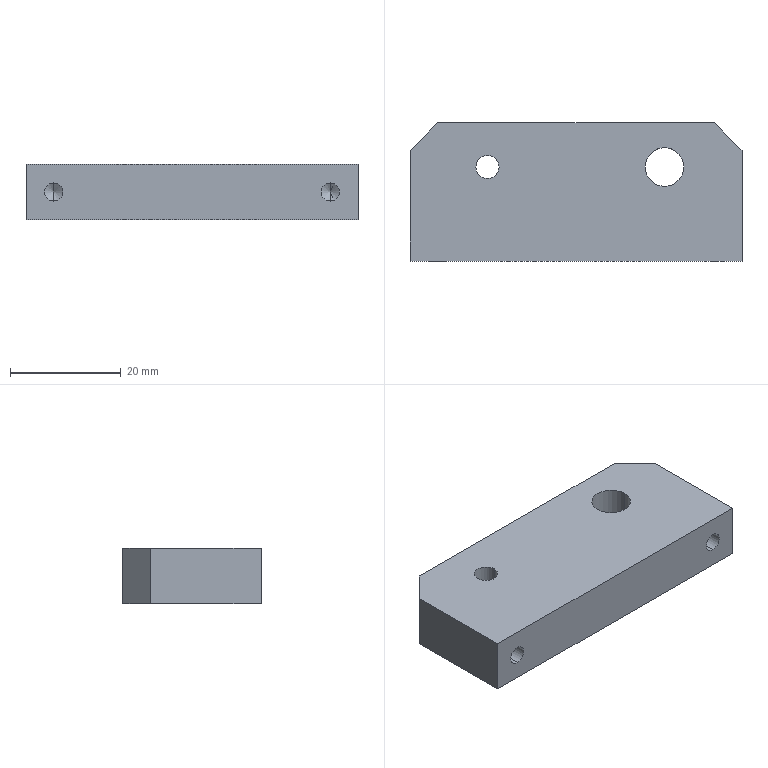Part | STEP file | PN_0049 Mount electronic clip cylinder mounting plate 2 | 1 solid | 20 faces | box 60 x 25 x 10 mm | volume 13990 mm3 | cylinder 8 | plane 8 | cone 4 | commonest cylinder face diameters 3.3 x4 4.2 x2 7 x2
STEP:
#1=CARTESIAN_POINT('',(0.,0.,0.));
#2=DIRECTION('',(0.,0.,1.));
#3=DIRECTION('',(1.,0.,0.));
#4=AXIS2_PLACEMENT_3D('',#1,#2,#3);
#5=CARTESIAN_POINT('',(-18.1,4.5,10.));
#6=VERTEX_POINT('',#5);
#7=CARTESIAN_POINT('',(-18.1,4.5,0.));
#8=VERTEX_POINT('',#7);
#9=CARTESIAN_POINT('',(-18.1,4.5,0.));
#10=DIRECTION('',(0.,0.,-1.));
#11=VECTOR('',#10,1.);
#12=LINE('',#9,#11);
#13=CARTESIAN_POINT('',(-16.,4.5,0.));
#14=DIRECTION('',(0.,0.,-1.));
#15=DIRECTION('',(-1.,0.,0.));
#16=AXIS2_PLACEMENT_3D('',#13,#14,#15);
#17=CYLINDRICAL_SURFACE('',#16,2.1);
#18=CARTESIAN_POINT('',(6.283,0.));
#19=DIRECTION('',(0.,1.));
#20=VECTOR('',#19,1.);
#21=LINE('',#18,#20);
#22=(GEOMETRIC_REPRESENTATION_CONTEXT(2)PARAMETRIC_REPRESENTATION_CONTEXT()REPRESENTATION_CONTEXT('',''));
#23=DEFINITIONAL_REPRESENTATION('',(#21),#22);
#24=PCURVE('',#17,#23);
#25=CARTESIAN_POINT('',(-16.,4.5,0.));
#26=DIRECTION('',(0.,0.,-1.));
#27=DIRECTION('',(-1.,0.,0.));
#28=AXIS2_PLACEMENT_3D('',#25,#26,#27);
#29=CYLINDRICAL_SURFACE('',#28,2.1);
#30=CARTESIAN_POINT('',(0.,0.));
#31=DIRECTION('',(0.,1.));
#32=VECTOR('',#31,1.);
#33=LINE('',#30,#32);
#34=(GEOMETRIC_REPRESENTATION_CONTEXT(2)PARAMETRIC_REPRESENTATION_CONTEXT()REPRESENTATION_CONTEXT('',''));
#35=DEFINITIONAL_REPRESENTATION('',(#33),#34);
#36=PCURVE('',#29,#35);
#37=SURFACE_CURVE('',#12,(#24,#36),.PCURVE_S1.);
#38=EDGE_CURVE('',#6,#8,#37,.T.);
#39=ORIENTED_EDGE('',*,*,#38,.T.);
#40=CARTESIAN_POINT('',(-13.9,4.5,0.));
#41=VERTEX_POINT('',#40);
#42=CARTESIAN_POINT('',(-16.,4.5,0.));
#43=DIRECTION('',(0.,0.,-1.));
#44=DIRECTION('',(-1.,0.,0.));
#45=AXIS2_PLACEMENT_3D('',#42,#43,#44);
#46=CIRCLE('',#45,2.1);
#47=CARTESIAN_POINT('',(0.,0.));
#48=DIRECTION('',(1.,0.));
#49=VECTOR('',#48,1.);
#50=LINE('',#47,#49);
#51=(GEOMETRIC_REPRESENTATION_CONTEXT(2)PARAMETRIC_REPRESENTATION_CONTEXT()REPRESENTATION_CONTEXT('',''));
#52=DEFINITIONAL_REPRESENTATION('',(#50),#51);
#53=PCURVE('',#17,#52);
#54=CARTESIAN_POINT('',(0.,0.,0.));
#55=DIRECTION('',(0.,0.,-1.));
#56=DIRECTION('',(-1.,0.,0.));
#57=AXIS2_PLACEMENT_3D('',#54,#55,#56);
#58=PLANE('',#57);
#59=CARTESIAN_POINT('',(16.,4.5));
#60=DIRECTION('',(1.,0.));
#61=AXIS2_PLACEMENT_2D('',#59,#60);
#62=CIRCLE('',#61,2.1);
#63=(GEOMETRIC_REPRESENTATION_CONTEXT(2)PARAMETRIC_REPRESENTATION_CONTEXT()REPRESENTATION_CONTEXT('',''));
#64=DEFINITIONAL_REPRESENTATION('',(#62),#63);
#65=PCURVE('',#58,#64);
#66=SURFACE_CURVE('',#46,(#53,#65),.PCURVE_S1.);
#67=EDGE_CURVE('',#41,#8,#66,.T.);
#68=ORIENTED_EDGE('',*,*,#67,.F.);
#69=CARTESIAN_POINT('',(-13.9,4.5,10.));
#70=VERTEX_POINT('',#69);
#71=CARTESIAN_POINT('',(-13.9,4.5,0.));
#72=DIRECTION('',(0.,0.,-1.));
#73=VECTOR('',#72,1.);
#74=LINE('',#71,#73);
#75=CARTESIAN_POINT('',(3.142,0.));
#76=DIRECTION('',(0.,1.));
#77=VECTOR('',#76,1.);
#78=LINE('',#75,#77);
#79=(GEOMETRIC_REPRESENTATION_CONTEXT(2)PARAMETRIC_REPRESENTATION_CONTEXT()REPRESENTATION_CONTEXT('',''));
#80=DEFINITIONAL_REPRESENTATION('',(#78),#79);
#81=PCURVE('',#17,#80);
#82=CARTESIAN_POINT('',(3.142,0.));
#83=DIRECTION('',(0.,1.));
#84=VECTOR('',#83,1.);
#85=LINE('',#82,#84);
#86=(GEOMETRIC_REPRESENTATION_CONTEXT(2)PARAMETRIC_REPRESENTATION_CONTEXT()REPRESENTATION_CONTEXT('',''));
#87=DEFINITIONAL_REPRESENTATION('',(#85),#86);
#88=PCURVE('',#29,#87);
#89=SURFACE_CURVE('',#74,(#81,#88),.PCURVE_S1.);
#90=EDGE_CURVE('',#70,#41,#89,.T.);
#91=ORIENTED_EDGE('',*,*,#90,.F.);
#92=CARTESIAN_POINT('',(-16.,4.5,10.));
#93=DIRECTION('',(0.,0.,-1.));
#94=DIRECTION('',(-1.,0.,0.));
#95=AXIS2_PLACEMENT_3D('',#92,#93,#94);
#96=CIRCLE('',#95,2.1);
#97=CARTESIAN_POINT('',(0.,-10.));
#98=DIRECTION('',(1.,0.));
#99=VECTOR('',#98,1.);
#100=LINE('',#97,#99);
#101=(GEOMETRIC_REPRESENTATION_CONTEXT(2)PARAMETRIC_REPRESENTATION_CONTEXT()REPRESENTATION_CONTEXT('',''));
#102=DEFINITIONAL_REPRESENTATION('',(#100),#101);
#103=PCURVE('',#17,#102);
#104=CARTESIAN_POINT('',(0.,0.,10.));
#105=DIRECTION('',(0.,0.,-1.));
#106=DIRECTION('',(-1.,0.,0.));
#107=AXIS2_PLACEMENT_3D('',#104,#105,#106);
#108=PLANE('',#107);
#109=CARTESIAN_POINT('',(16.,4.5));
#110=DIRECTION('',(1.,0.));
#111=AXIS2_PLACEMENT_2D('',#109,#110);
#112=CIRCLE('',#111,2.1);
#113=(GEOMETRIC_REPRESENTATION_CONTEXT(2)PARAMETRIC_REPRESENTATION_CONTEXT()REPRESENTATION_CONTEXT('',''));
#114=DEFINITIONAL_REPRESENTATION('',(#112),#113);
#115=PCURVE('',#108,#114);
#116=SURFACE_CURVE('',#96,(#103,#115),.PCURVE_S1.);
#117=EDGE_CURVE('',#70,#6,#116,.T.);
#118=ORIENTED_EDGE('',*,*,#117,.T.);
#119=EDGE_LOOP('',(#39,#68,#91,#118));
#120=FACE_BOUND('',#119,.F.);
#121=ADVANCED_FACE('',(#120),#17,.F.);
#122=CARTESIAN_POINT('',(12.5,4.5,10.));
#123=VERTEX_POINT('',#122);
#124=CARTESIAN_POINT('',(12.5,4.5,0.));
#125=VERTEX_POINT('',#124);
#126=CARTESIAN_POINT('',(12.5,4.5,0.));
#127=DIRECTION('',(0.,0.,-1.));
#128=VECTOR('',#127,1.);
#129=LINE('',#126,#128);
#130=CARTESIAN_POINT('',(16.,4.5,0.));
#131=DIRECTION('',(0.,0.,-1.));
#132=DIRECTION('',(-1.,0.,0.));
#133=AXIS2_PLACEMENT_3D('',#130,#131,#132);
#134=CYLINDRICAL_SURFACE('',#133,3.5);
#135=CARTESIAN_POINT('',(6.283,0.));
#136=DIRECTION('',(0.,1.));
#137=VECTOR('',#136,1.);
#138=LINE('',#135,#137);
#139=(GEOMETRIC_REPRESENTATION_CONTEXT(2)PARAMETRIC_REPRESENTATION_CONTEXT()REPRESENTATION_CONTEXT('',''));
#140=DEFINITIONAL_REPRESENTATION('',(#138),#139);
#141=PCURVE('',#134,#140);
#142=CARTESIAN_POINT('',(16.,4.5,0.));
#143=DIRECTION('',(0.,0.,-1.));
#144=DIRECTION('',(-1.,0.,0.));
#145=AXIS2_PLACEMENT_3D('',#142,#143,#144);
#146=CYLINDRICAL_SURFACE('',#145,3.5);
#147=CARTESIAN_POINT('',(0.,0.));
#148=DIRECTION('',(0.,1.));
#149=VECTOR('',#148,1.);
#150=LINE('',#147,#149);
#151=(GEOMETRIC_REPRESENTATION_CONTEXT(2)PARAMETRIC_REPRESENTATION_CONTEXT()REPRESENTATION_CONTEXT('',''));
#152=DEFINITIONAL_REPRESENTATION('',(#150),#151);
#153=PCURVE('',#146,#152);
#154=SURFACE_CURVE('',#129,(#141,#153),.PCURVE_S1.);
#155=EDGE_CURVE('',#123,#125,#154,.T.);
#156=ORIENTED_EDGE('',*,*,#155,.T.);
#157=CARTESIAN_POINT('',(19.5,4.5,0.));
#158=VERTEX_POINT('',#157);
#159=CARTESIAN_POINT('',(16.,4.5,0.));
#160=DIRECTION('',(0.,0.,-1.));
#161=DIRECTION('',(-1.,0.,0.));
#162=AXIS2_PLACEMENT_3D('',#159,#160,#161);
#163=CIRCLE('',#162,3.5);
#164=CARTESIAN_POINT('',(0.,0.));
#165=DIRECTION('',(1.,0.));
#166=VECTOR('',#165,1.);
#167=LINE('',#164,#166);
#168=(GEOMETRIC_REPRESENTATION_CONTEXT(2)PARAMETRIC_REPRESENTATION_CONTEXT()REPRESENTATION_CONTEXT('',''));
#169=DEFINITIONAL_REPRESENTATION('',(#167),#168);
#170=PCURVE('',#134,#169);
#171=CARTESIAN_POINT('',(-16.,4.5));
#172=DIRECTION('',(1.,0.));
#173=AXIS2_PLACEMENT_2D('',#171,#172);
#174=CIRCLE('',#173,3.5);
#175=(GEOMETRIC_REPRESENTATION_CONTEXT(2)PARAMETRIC_REPRESENTATION_CONTEXT()REPRESENTATION_CONTEXT('',''));
#176=DEFINITIONAL_REPRESENTATION('',(#174),#175);
#177=PCURVE('',#58,#176);
#178=SURFACE_CURVE('',#163,(#170,#177),.PCURVE_S1.);
#179=EDGE_CURVE('',#158,#125,#178,.T.);
#180=ORIENTED_EDGE('',*,*,#179,.F.);
#181=CARTESIAN_POINT('',(19.5,4.5,10.));
#182=VERTEX_POINT('',#181);
#183=CARTESIAN_POINT('',(19.5,4.5,0.));
#184=DIRECTION('',(0.,0.,-1.));
#185=VECTOR('',#184,1.);
#186=LINE('',#183,#185);
#187=CARTESIAN_POINT('',(3.142,0.));
#188=DIRECTION('',(0.,1.));
#189=VECTOR('',#188,1.);
#190=LINE('',#187,#189);
#191=(GEOMETRIC_REPRESENTATION_CONTEXT(2)PARAMETRIC_REPRESENTATION_CONTEXT()REPRESENTATION_CONTEXT('',''));
#192=DEFINITIONAL_REPRESENTATION('',(#190),#191);
#193=PCURVE('',#134,#192);
#194=CARTESIAN_POINT('',(3.142,0.));
#195=DIRECTION('',(0.,1.));
#196=VECTOR('',#195,1.);
#197=LINE('',#194,#196);
#198=(GEOMETRIC_REPRESENTATION_CONTEXT(2)PARAMETRIC_REPRESENTATION_CONTEXT()REPRESENTATION_CONTEXT('',''));
#199=DEFINITIONAL_REPRESENTATION('',(#197),#198);
#200=PCURVE('',#146,#199);
#201=SURFACE_CURVE('',#186,(#193,#200),.PCURVE_S1.);
#202=EDGE_CURVE('',#182,#158,#201,.T.);
#203=ORIENTED_EDGE('',*,*,#202,.F.);
#204=CARTESIAN_POINT('',(16.,4.5,10.));
#205=DIRECTION('',(0.,0.,-1.));
#206=DIRECTION('',(-1.,0.,0.));
#207=AXIS2_PLACEMENT_3D('',#204,#205,#206);
#208=CIRCLE('',#207,3.5);
#209=CARTESIAN_POINT('',(0.,-10.));
#210=DIRECTION('',(1.,0.));
#211=VECTOR('',#210,1.);
#212=LINE('',#209,#211);
#213=(GEOMETRIC_REPRESENTATION_CONTEXT(2)PARAMETRIC_REPRESENTATION_CONTEXT()REPRESENTATION_CONTEXT('',''));
#214=DEFINITIONAL_REPRESENTATION('',(#212),#213);
#215=PCURVE('',#134,#214);
#216=CARTESIAN_POINT('',(-16.,4.5));
#217=DIRECTION('',(1.,0.));
#218=AXIS2_PLACEMENT_2D('',#216,#217);
#219=CIRCLE('',#218,3.5);
#220=(GEOMETRIC_REPRESENTATION_CONTEXT(2)PARAMETRIC_REPRESENTATION_CONTEXT()REPRESENTATION_CONTEXT('',''));
#221=DEFINITIONAL_REPRESENTATION('',(#219),#220);
#222=PCURVE('',#108,#221);
#223=SURFACE_CURVE('',#208,(#215,#222),.PCURVE_S1.);
#224=EDGE_CURVE('',#182,#123,#223,.T.);
#225=ORIENTED_EDGE('',*,*,#224,.T.);
#226=EDGE_LOOP('',(#156,#180,#203,#225));
#227=FACE_BOUND('',#226,.F.);
#228=ADVANCED_FACE('',(#227),#134,.F.);
#229=CARTESIAN_POINT('',(25.,1.,3.35));
#230=VERTEX_POINT('',#229);
#231=CARTESIAN_POINT('',(25.,-12.5,3.35));
#232=VERTEX_POINT('',#231);
#233=CARTESIAN_POINT('',(25.,-12.5,3.35));
#234=DIRECTION('',(0.,-1.,0.));
#235=VECTOR('',#234,1.);
#236=LINE('',#233,#235);
#237=CARTESIAN_POINT('',(25.,-12.5,5.));
#238=DIRECTION('',(0.,-1.,0.));
#239=DIRECTION('',(0.,0.,-1.));
#240=AXIS2_PLACEMENT_3D('',#237,#238,#239);
#241=CYLINDRICAL_SURFACE('',#240,1.65);
#242=CARTESIAN_POINT('',(6.283,0.));
#243=DIRECTION('',(0.,1.));
#244=VECTOR('',#243,1.);
#245=LINE('',#242,#244);
#246=(GEOMETRIC_REPRESENTATION_CONTEXT(2)PARAMETRIC_REPRESENTATION_CONTEXT()REPRESENTATION_CONTEXT('',''));
#247=DEFINITIONAL_REPRESENTATION('',(#245),#246);
#248=PCURVE('',#241,#247);
#249=CARTESIAN_POINT('',(25.,-12.5,5.));
#250=DIRECTION('',(0.,-1.,0.));
#251=DIRECTION('',(0.,0.,-1.));
#252=AXIS2_PLACEMENT_3D('',#249,#250,#251);
#253=CYLINDRICAL_SURFACE('',#252,1.65);
#254=CARTESIAN_POINT('',(0.,0.));
#255=DIRECTION('',(0.,1.));
#256=VECTOR('',#255,1.);
#257=LINE('',#254,#256);
#258=(GEOMETRIC_REPRESENTATION_CONTEXT(2)PARAMETRIC_REPRESENTATION_CONTEXT()REPRESENTATION_CONTEXT('',''));
#259=DEFINITIONAL_REPRESENTATION('',(#257),#258);
#260=PCURVE('',#253,#259);
#261=SURFACE_CURVE('',#236,(#248,#260),.PCURVE_S1.);
#262=EDGE_CURVE('',#230,#232,#261,.T.);
#263=ORIENTED_EDGE('',*,*,#262,.T.);
#264=CARTESIAN_POINT('',(25.,-12.5,6.65));
#265=VERTEX_POINT('',#264);
#266=CARTESIAN_POINT('',(25.,-12.5,5.));
#267=DIRECTION('',(0.,-1.,0.));
#268=DIRECTION('',(0.,0.,-1.));
#269=AXIS2_PLACEMENT_3D('',#266,#267,#268);
#270=CIRCLE('',#269,1.65);
#271=CARTESIAN_POINT('',(0.,0.));
#272=DIRECTION('',(1.,0.));
#273=VECTOR('',#272,1.);
#274=LINE('',#271,#273);
#275=(GEOMETRIC_REPRESENTATION_CONTEXT(2)PARAMETRIC_REPRESENTATION_CONTEXT()REPRESENTATION_CONTEXT('',''));
#276=DEFINITIONAL_REPRESENTATION('',(#274),#275);
#277=PCURVE('',#241,#276);
#278=CARTESIAN_POINT('',(-30.,-12.5,10.));
#279=DIRECTION('',(0.,1.,0.));
#280=DIRECTION('',(0.,0.,1.));
#281=AXIS2_PLACEMENT_3D('',#278,#279,#280);
#282=PLANE('',#281);
#283=CARTESIAN_POINT('',(-6.65,55.));
#284=CARTESIAN_POINT('',(-6.65,57.858));
#285=CARTESIAN_POINT('',(-4.175,56.429));
#286=CARTESIAN_POINT('',(-1.7,55.));
#287=CARTESIAN_POINT('',(-4.175,53.571));
#288=CARTESIAN_POINT('',(-6.65,52.142));
#289=CARTESIAN_POINT('',(-6.65,55.));
#290=(BOUNDED_CURVE()B_SPLINE_CURVE(2,(#283,#284,#285,#286,#287,#288,#289),.UNSPECIFIED.,.T.,.F.)B_SPLINE_CURVE_WITH_KNOTS((1,2,2,2,2,1),(-2.094,0.,2.094,4.189,6.283,8.378),.UNSPECIFIED.)CURVE()GEOMETRIC_REPRESENTATION_ITEM()RATIONAL_B_SPLINE_CURVE((1.,0.5,1.,0.5,1.,0.5,1.))REPRESENTATION_ITEM(''));
#291=(GEOMETRIC_REPRESENTATION_CONTEXT(2)PARAMETRIC_REPRESENTATION_CONTEXT()REPRESENTATION_CONTEXT('',''));
#292=DEFINITIONAL_REPRESENTATION('',(#290),#291);
#293=PCURVE('',#282,#292);
#294=SURFACE_CURVE('',#270,(#277,#293),.PCURVE_S1.);
#295=EDGE_CURVE('',#265,#232,#294,.T.);
#296=ORIENTED_EDGE('',*,*,#295,.F.);
#297=CARTESIAN_POINT('',(25.,1.,6.65));
#298=VERTEX_POINT('',#297);
#299=CARTESIAN_POINT('',(25.,-12.5,6.65));
#300=DIRECTION('',(0.,-1.,0.));
#301=VECTOR('',#300,1.);
#302=LINE('',#299,#301);
#303=CARTESIAN_POINT('',(3.142,0.));
#304=DIRECTION('',(0.,1.));
#305=VECTOR('',#304,1.);
#306=LINE('',#303,#305);
#307=(GEOMETRIC_REPRESENTATION_CONTEXT(2)PARAMETRIC_REPRESENTATION_CONTEXT()REPRESENTATION_CONTEXT('',''));
#308=DEFINITIONAL_REPRESENTATION('',(#306),#307);
#309=PCURVE('',#241,#308);
#310=CARTESIAN_POINT('',(3.142,0.));
#311=DIRECTION('',(0.,1.));
#312=VECTOR('',#311,1.);
#313=LINE('',#310,#312);
#314=(GEOMETRIC_REPRESENTATION_CONTEXT(2)PARAMETRIC_REPRESENTATION_CONTEXT()REPRESENTATION_CONTEXT('',''));
#315=DEFINITIONAL_REPRESENTATION('',(#313),#314);
#316=PCURVE('',#253,#315);
#317=SURFACE_CURVE('',#302,(#309,#316),.PCURVE_S1.);
#318=EDGE_CURVE('',#298,#265,#317,.T.);
#319=ORIENTED_EDGE('',*,*,#318,.F.);
#320=CARTESIAN_POINT('',(25.,1.,5.));
#321=DIRECTION('',(0.,-1.,0.));
#322=DIRECTION('',(0.,0.,-1.));
#323=AXIS2_PLACEMENT_3D('',#320,#321,#322);
#324=CIRCLE('',#323,1.65);
#325=CARTESIAN_POINT('',(0.,-13.5));
#326=DIRECTION('',(1.,0.));
#327=VECTOR('',#326,1.);
#328=LINE('',#325,#327);
#329=(GEOMETRIC_REPRESENTATION_CONTEXT(2)PARAMETRIC_REPRESENTATION_CONTEXT()REPRESENTATION_CONTEXT('',''));
#330=DEFINITIONAL_REPRESENTATION('',(#328),#329);
#331=PCURVE('',#241,#330);
#332=CARTESIAN_POINT('',(25.,1.,5.));
#333=DIRECTION('',(0.,-1.,0.));
#334=DIRECTION('',(0.,0.,-1.));
#335=AXIS2_PLACEMENT_3D('',#332,#333,#334);
#336=CONICAL_SURFACE('',#335,1.65,1.03);
#337=CARTESIAN_POINT('',(0.,0.));
#338=DIRECTION('',(1.,0.));
#339=VECTOR('',#338,1.);
#340=LINE('',#337,#339);
#341=(GEOMETRIC_REPRESENTATION_CONTEXT(2)PARAMETRIC_REPRESENTATION_CONTEXT()REPRESENTATION_CONTEXT('',''));
#342=DEFINITIONAL_REPRESENTATION('',(#340),#341);
#343=PCURVE('',#336,#342);
#344=SURFACE_CURVE('',#324,(#331,#343),.PCURVE_S1.);
#345=EDGE_CURVE('',#298,#230,#344,.T.);
#346=ORIENTED_EDGE('',*,*,#345,.T.);
#347=EDGE_LOOP('',(#263,#296,#319,#346));
#348=FACE_BOUND('',#347,.F.);
#349=ADVANCED_FACE('',(#348),#241,.F.);
#350=ORIENTED_EDGE('',*,*,#345,.F.);
#351=CARTESIAN_POINT('',(25.,1.991,5.));
#352=VERTEX_POINT('',#351);
#353=CARTESIAN_POINT('',(25.,1.,6.65));
#354=DIRECTION('',(0.,-0.515,0.8572));
#355=VECTOR('',#354,1.);
#356=LINE('',#353,#355);
#357=CARTESIAN_POINT('',(3.142,0.));
#358=DIRECTION('',(0.,1.));
#359=VECTOR('',#358,1.);
#360=LINE('',#357,#359);
#361=(GEOMETRIC_REPRESENTATION_CONTEXT(2)PARAMETRIC_REPRESENTATION_CONTEXT()REPRESENTATION_CONTEXT('',''));
#362=DEFINITIONAL_REPRESENTATION('',(#360),#361);
#363=PCURVE('',#336,#362);
#364=CARTESIAN_POINT('',(25.,1.,5.));
#365=DIRECTION('',(0.,-1.,0.));
#366=DIRECTION('',(0.,0.,-1.));
#367=AXIS2_PLACEMENT_3D('',#364,#365,#366);
#368=CONICAL_SURFACE('',#367,1.65,1.03);
#369=CARTESIAN_POINT('',(3.142,0.));
#370=DIRECTION('',(0.,1.));
#371=VECTOR('',#370,1.);
#372=LINE('',#369,#371);
#373=(GEOMETRIC_REPRESENTATION_CONTEXT(2)PARAMETRIC_REPRESENTATION_CONTEXT()REPRESENTATION_CONTEXT('',''));
#374=DEFINITIONAL_REPRESENTATION('',(#372),#373);
#375=PCURVE('',#368,#374);
#376=SURFACE_CURVE('',#356,(#363,#375),.PCURVE_S1.);
#377=EDGE_CURVE('',#352,#298,#376,.T.);
#378=ORIENTED_EDGE('',*,*,#377,.F.);
#379=CARTESIAN_POINT('',(25.,1.,3.35));
#380=DIRECTION('',(0.,-0.515,-0.8572));
#381=VECTOR('',#380,1.);
#382=LINE('',#379,#381);
#383=CARTESIAN_POINT('',(6.283,0.));
#384=DIRECTION('',(0.,1.));
#385=VECTOR('',#384,1.);
#386=LINE('',#383,#385);
#387=(GEOMETRIC_REPRESENTATION_CONTEXT(2)PARAMETRIC_REPRESENTATION_CONTEXT()REPRESENTATION_CONTEXT('',''));
#388=DEFINITIONAL_REPRESENTATION('',(#386),#387);
#389=PCURVE('',#336,#388);
#390=CARTESIAN_POINT('',(0.,0.));
#391=DIRECTION('',(0.,1.));
#392=VECTOR('',#391,1.);
#393=LINE('',#390,#392);
#394=(GEOMETRIC_REPRESENTATION_CONTEXT(2)PARAMETRIC_REPRESENTATION_CONTEXT()REPRESENTATION_CONTEXT('',''));
#395=DEFINITIONAL_REPRESENTATION('',(#393),#394);
#396=PCURVE('',#368,#395);
#397=SURFACE_CURVE('',#382,(#389,#396),.PCURVE_S1.);
#398=EDGE_CURVE('',#352,#230,#397,.T.);
#399=ORIENTED_EDGE('',*,*,#398,.T.);
#400=EDGE_LOOP('',(#350,#378,#399));
#401=FACE_BOUND('',#400,.F.);
#402=ADVANCED_FACE('',(#401),#336,.F.);
#403=CARTESIAN_POINT('',(-25.,1.,3.35));
#404=VERTEX_POINT('',#403);
#405=CARTESIAN_POINT('',(-25.,-12.5,3.35));
#406=VERTEX_POINT('',#405);
#407=CARTESIAN_POINT('',(-25.,-12.5,3.35));
#408=DIRECTION('',(0.,-1.,0.));
#409=VECTOR('',#408,1.);
#410=LINE('',#407,#409);
#411=CARTESIAN_POINT('',(-25.,-12.5,5.));
#412=DIRECTION('',(0.,-1.,0.));
#413=DIRECTION('',(0.,0.,-1.));
#414=AXIS2_PLACEMENT_3D('',#411,#412,#413);
#415=CYLINDRICAL_SURFACE('',#414,1.65);
#416=CARTESIAN_POINT('',(6.283,0.));
#417=DIRECTION('',(0.,1.));
#418=VECTOR('',#417,1.);
#419=LINE('',#416,#418);
#420=(GEOMETRIC_REPRESENTATION_CONTEXT(2)PARAMETRIC_REPRESENTATION_CONTEXT()REPRESENTATION_CONTEXT('',''));
#421=DEFINITIONAL_REPRESENTATION('',(#419),#420);
#422=PCURVE('',#415,#421);
#423=CARTESIAN_POINT('',(-25.,-12.5,5.));
#424=DIRECTION('',(0.,-1.,0.));
#425=DIRECTION('',(0.,0.,-1.));
#426=AXIS2_PLACEMENT_3D('',#423,#424,#425);
#427=CYLINDRICAL_SURFACE('',#426,1.65);
#428=CARTESIAN_POINT('',(0.,0.));
#429=DIRECTION('',(0.,1.));
#430=VECTOR('',#429,1.);
#431=LINE('',#428,#430);
#432=(GEOMETRIC_REPRESENTATION_CONTEXT(2)PARAMETRIC_REPRESENTATION_CONTEXT()REPRESENTATION_CONTEXT('',''));
#433=DEFINITIONAL_REPRESENTATION('',(#431),#432);
#434=PCURVE('',#427,#433);
#435=SURFACE_CURVE('',#410,(#422,#434),.PCURVE_S1.);
#436=EDGE_CURVE('',#404,#406,#435,.T.);
#437=ORIENTED_EDGE('',*,*,#436,.T.);
#438=CARTESIAN_POINT('',(-25.,-12.5,6.65));
#439=VERTEX_POINT('',#438);
#440=CARTESIAN_POINT('',(-25.,-12.5,5.));
#441=DIRECTION('',(0.,-1.,0.));
#442=DIRECTION('',(0.,0.,-1.));
#443=AXIS2_PLACEMENT_3D('',#440,#441,#442);
#444=CIRCLE('',#443,1.65);
#445=CARTESIAN_POINT('',(0.,0.));
#446=DIRECTION('',(1.,0.));
#447=VECTOR('',#446,1.);
#448=LINE('',#445,#447);
#449=(GEOMETRIC_REPRESENTATION_CONTEXT(2)PARAMETRIC_REPRESENTATION_CONTEXT()REPRESENTATION_CONTEXT('',''));
#450=DEFINITIONAL_REPRESENTATION('',(#448),#449);
#451=PCURVE('',#415,#450);
#452=CARTESIAN_POINT('',(-6.65,5.));
#453=CARTESIAN_POINT('',(-6.65,7.858));
#454=CARTESIAN_POINT('',(-4.175,6.429));
#455=CARTESIAN_POINT('',(-1.7,5.));
#456=CARTESIAN_POINT('',(-4.175,3.571));
#457=CARTESIAN_POINT('',(-6.65,2.142));
#458=CARTESIAN_POINT('',(-6.65,5.));
#459=(BOUNDED_CURVE()B_SPLINE_CURVE(2,(#452,#453,#454,#455,#456,#457,#458),.UNSPECIFIED.,.T.,.F.)B_SPLINE_CURVE_WITH_KNOTS((1,2,2,2,2,1),(-2.094,0.,2.094,4.189,6.283,8.378),.UNSPECIFIED.)CURVE()GEOMETRIC_REPRESENTATION_ITEM()RATIONAL_B_SPLINE_CURVE((1.,0.5,1.,0.5,1.,0.5,1.))REPRESENTATION_ITEM(''));
#460=(GEOMETRIC_REPRESENTATION_CONTEXT(2)PARAMETRIC_REPRESENTATION_CONTEXT()REPRESENTATION_CONTEXT('',''));
#461=DEFINITIONAL_REPRESENTATION('',(#459),#460);
#462=PCURVE('',#282,#461);
#463=SURFACE_CURVE('',#444,(#451,#462),.PCURVE_S1.);
#464=EDGE_CURVE('',#439,#406,#463,.T.);
#465=ORIENTED_EDGE('',*,*,#464,.F.);
#466=CARTESIAN_POINT('',(-25.,1.,6.65));
#467=VERTEX_POINT('',#466);
#468=CARTESIAN_POINT('',(-25.,-12.5,6.65));
#469=DIRECTION('',(0.,-1.,0.));
#470=VECTOR('',#469,1.);
#471=LINE('',#468,#470);
#472=CARTESIAN_POINT('',(3.142,0.));
#473=DIRECTION('',(0.,1.));
#474=VECTOR('',#473,1.);
#475=LINE('',#472,#474);
#476=(GEOMETRIC_REPRESENTATION_CONTEXT(2)PARAMETRIC_REPRESENTATION_CONTEXT()REPRESENTATION_CONTEXT('',''));
#477=DEFINITIONAL_REPRESENTATION('',(#475),#476);
#478=PCURVE('',#415,#477);
#479=CARTESIAN_POINT('',(3.142,0.));
#480=DIRECTION('',(0.,1.));
#481=VECTOR('',#480,1.);
#482=LINE('',#479,#481);
#483=(GEOMETRIC_REPRESENTATION_CONTEXT(2)PARAMETRIC_REPRESENTATION_CONTEXT()REPRESENTATION_CONTEXT('',''));
#484=DEFINITIONAL_REPRESENTATION('',(#482),#483);
#485=PCURVE('',#427,#484);
#486=SURFACE_CURVE('',#471,(#478,#485),.PCURVE_S1.);
#487=EDGE_CURVE('',#467,#439,#486,.T.);
#488=ORIENTED_EDGE('',*,*,#487,.F.);
#489=CARTESIAN_POINT('',(-25.,1.,5.));
#490=DIRECTION('',(0.,-1.,0.));
#491=DIRECTION('',(0.,0.,-1.));
#492=AXIS2_PLACEMENT_3D('',#489,#490,#491);
#493=CIRCLE('',#492,1.65);
#494=CARTESIAN_POINT('',(0.,-13.5));
#495=DIRECTION('',(1.,0.));
#496=VECTOR('',#495,1.);
#497=LINE('',#494,#496);
#498=(GEOMETRIC_REPRESENTATION_CONTEXT(2)PARAMETRIC_REPRESENTATION_CONTEXT()REPRESENTATION_CONTEXT('',''));
#499=DEFINITIONAL_REPRESENTATION('',(#497),#498);
#500=PCURVE('',#415,#499);
#501=CARTESIAN_POINT('',(-25.,1.,5.));
#502=DIRECTION('',(0.,-1.,0.));
#503=DIRECTION('',(0.,0.,-1.));
#504=AXIS2_PLACEMENT_3D('',#501,#502,#503);
#505=CONICAL_SURFACE('',#504,1.65,1.03);
#506=CARTESIAN_POINT('',(0.,0.));
#507=DIRECTION('',(1.,0.));
#508=VECTOR('',#507,1.);
#509=LINE('',#506,#508);
#510=(GEOMETRIC_REPRESENTATION_CONTEXT(2)PARAMETRIC_REPRESENTATION_CONTEXT()REPRESENTATION_CONTEXT('',''));
#511=DEFINITIONAL_REPRESENTATION('',(#509),#510);
#512=PCURVE('',#505,#511);
#513=SURFACE_CURVE('',#493,(#500,#512),.PCURVE_S1.);
#514=EDGE_CURVE('',#467,#404,#513,.T.);
#515=ORIENTED_EDGE('',*,*,#514,.T.);
#516=EDGE_LOOP('',(#437,#465,#488,#515));
#517=FACE_BOUND('',#516,.F.);
#518=ADVANCED_FACE('',(#517),#415,.F.);
#519=ORIENTED_EDGE('',*,*,#514,.F.);
#520=CARTESIAN_POINT('',(-25.,1.991,5.));
#521=VERTEX_POINT('',#520);
#522=CARTESIAN_POINT('',(-25.,1.,6.65));
#523=DIRECTION('',(0.,-0.515,0.8572));
#524=VECTOR('',#523,1.);
#525=LINE('',#522,#524);
#526=CARTESIAN_POINT('',(3.142,0.));
#527=DIRECTION('',(0.,1.));
#528=VECTOR('',#527,1.);
#529=LINE('',#526,#528);
#530=(GEOMETRIC_REPRESENTATION_CONTEXT(2)PARAMETRIC_REPRESENTATION_CONTEXT()REPRESENTATION_CONTEXT('',''));
#531=DEFINITIONAL_REPRESENTATION('',(#529),#530);
#532=PCURVE('',#505,#531);
#533=CARTESIAN_POINT('',(-25.,1.,5.));
#534=DIRECTION('',(0.,-1.,0.));
#535=DIRECTION('',(0.,0.,-1.));
#536=AXIS2_PLACEMENT_3D('',#533,#534,#535);
#537=CONICAL_SURFACE('',#536,1.65,1.03);
#538=CARTESIAN_POINT('',(3.142,0.));
#539=DIRECTION('',(0.,1.));
#540=VECTOR('',#539,1.);
#541=LINE('',#538,#540);
#542=(GEOMETRIC_REPRESENTATION_CONTEXT(2)PARAMETRIC_REPRESENTATION_CONTEXT()REPRESENTATION_CONTEXT('',''));
#543=DEFINITIONAL_REPRESENTATION('',(#541),#542);
#544=PCURVE('',#537,#543);
#545=SURFACE_CURVE('',#525,(#532,#544),.PCURVE_S1.);
#546=EDGE_CURVE('',#521,#467,#545,.T.);
#547=ORIENTED_EDGE('',*,*,#546,.F.);
#548=CARTESIAN_POINT('',(-25.,1.,3.35));
#549=DIRECTION('',(0.,-0.515,-0.8572));
#550=VECTOR('',#549,1.);
#551=LINE('',#548,#550);
#552=CARTESIAN_POINT('',(6.283,0.));
#553=DIRECTION('',(0.,1.));
#554=VECTOR('',#553,1.);
#555=LINE('',#552,#554);
#556=(GEOMETRIC_REPRESENTATION_CONTEXT(2)PARAMETRIC_REPRESENTATION_CONTEXT()REPRESENTATION_CONTEXT('',''));
#557=DEFINITIONAL_REPRESENTATION('',(#555),#556);
#558=PCURVE('',#505,#557);
#559=CARTESIAN_POINT('',(0.,0.));
#560=DIRECTION('',(0.,1.));
#561=VECTOR('',#560,1.);
#562=LINE('',#559,#561);
#563=(GEOMETRIC_REPRESENTATION_CONTEXT(2)PARAMETRIC_REPRESENTATION_CONTEXT()REPRESENTATION_CONTEXT('',''));
#564=DEFINITIONAL_REPRESENTATION('',(#562),#563);
#565=PCURVE('',#537,#564);
#566=SURFACE_CURVE('',#551,(#558,#565),.PCURVE_S1.);
#567=EDGE_CURVE('',#521,#404,#566,.T.);
#568=ORIENTED_EDGE('',*,*,#567,.T.);
#569=EDGE_LOOP('',(#519,#547,#568));
#570=FACE_BOUND('',#569,.F.);
#571=ADVANCED_FACE('',(#570),#505,.F.);
#572=CARTESIAN_POINT('',(30.,-12.5,0.));
#573=VERTEX_POINT('',#572);
#574=CARTESIAN_POINT('',(30.,7.5,0.));
#575=VERTEX_POINT('',#574);
#576=CARTESIAN_POINT('',(30.,-12.5,0.));
#577=DIRECTION('',(0.,1.,0.));
#578=VECTOR('',#577,1.);
#579=LINE('',#576,#578);
#580=CARTESIAN_POINT('',(30.,-12.5,10.));
#581=DIRECTION('',(-1.,0.,0.));
#582=DIRECTION('',(0.,0.,1.));
#583=AXIS2_PLACEMENT_3D('',#580,#581,#582);
#584=PLANE('',#583);
#585=CARTESIAN_POINT('',(-10.,0.));
#586=DIRECTION('',(0.,1.));
#587=VECTOR('',#586,1.);
#588=LINE('',#585,#587);
#589=(GEOMETRIC_REPRESENTATION_CONTEXT(2)PARAMETRIC_REPRESENTATION_CONTEXT()REPRESENTATION_CONTEXT('',''));
#590=DEFINITIONAL_REPRESENTATION('',(#588),#589);
#591=PCURVE('',#584,#590);
#592=CARTESIAN_POINT('',(-30.,-12.5));
#593=DIRECTION('',(0.,1.));
#594=VECTOR('',#593,1.);
#595=LINE('',#592,#594);
#596=(GEOMETRIC_REPRESENTATION_CONTEXT(2)PARAMETRIC_REPRESENTATION_CONTEXT()REPRESENTATION_CONTEXT('',''));
#597=DEFINITIONAL_REPRESENTATION('',(#595),#596);
#598=PCURVE('',#58,#597);
#599=SURFACE_CURVE('',#579,(#591,#598),.PCURVE_S1.);
#600=EDGE_CURVE('',#573,#575,#599,.T.);
#601=ORIENTED_EDGE('',*,*,#600,.T.);
#602=CARTESIAN_POINT('',(30.,7.5,10.));
#603=VERTEX_POINT('',#602);
#604=CARTESIAN_POINT('',(30.,7.5,10.));
#605=DIRECTION('',(0.,0.,1.));
#606=VECTOR('',#605,1.);
#607=LINE('',#604,#606);
#608=CARTESIAN_POINT('',(0.,20.));
#609=DIRECTION('',(1.,0.));
#610=VECTOR('',#609,1.);
#611=LINE('',#608,#610);
#612=(GEOMETRIC_REPRESENTATION_CONTEXT(2)PARAMETRIC_REPRESENTATION_CONTEXT()REPRESENTATION_CONTEXT('',''));
#613=DEFINITIONAL_REPRESENTATION('',(#611),#612);
#614=PCURVE('',#584,#613);
#615=CARTESIAN_POINT('',(25.,12.5,10.));
#616=DIRECTION('',(-0.7071,-0.7071,0.));
#617=DIRECTION('',(0.,0.,-1.));
#618=AXIS2_PLACEMENT_3D('',#615,#616,#617);
#619=PLANE('',#618);
#620=CARTESIAN_POINT('',(0.,7.071));
#621=DIRECTION('',(-1.,0.));
#622=VECTOR('',#621,1.);
#623=LINE('',#620,#622);
#624=(GEOMETRIC_REPRESENTATION_CONTEXT(2)PARAMETRIC_REPRESENTATION_CONTEXT()REPRESENTATION_CONTEXT('',''));
#625=DEFINITIONAL_REPRESENTATION('',(#623),#624);
#626=PCURVE('',#619,#625);
#627=SURFACE_CURVE('',#607,(#614,#626),.PCURVE_S1.);
#628=EDGE_CURVE('',#575,#603,#627,.T.);
#629=ORIENTED_EDGE('',*,*,#628,.T.);
#630=CARTESIAN_POINT('',(30.,-12.5,10.));
#631=VERTEX_POINT('',#630);
#632=CARTESIAN_POINT('',(30.,-12.5,10.));
#633=DIRECTION('',(0.,1.,0.));
#634=VECTOR('',#633,1.);
#635=LINE('',#632,#634);
#636=CARTESIAN_POINT('',(0.,0.));
#637=DIRECTION('',(0.,1.));
#638=VECTOR('',#637,1.);
#639=LINE('',#636,#638);
#640=(GEOMETRIC_REPRESENTATION_CONTEXT(2)PARAMETRIC_REPRESENTATION_CONTEXT()REPRESENTATION_CONTEXT('',''));
#641=DEFINITIONAL_REPRESENTATION('',(#639),#640);
#642=PCURVE('',#584,#641);
#643=CARTESIAN_POINT('',(-30.,-12.5));
#644=DIRECTION('',(0.,1.));
#645=VECTOR('',#644,1.);
#646=LINE('',#643,#645);
#647=(GEOMETRIC_REPRESENTATION_CONTEXT(2)PARAMETRIC_REPRESENTATION_CONTEXT()REPRESENTATION_CONTEXT('',''));
#648=DEFINITIONAL_REPRESENTATION('',(#646),#647);
#649=PCURVE('',#108,#648);
#650=SURFACE_CURVE('',#635,(#642,#649),.PCURVE_S1.);
#651=EDGE_CURVE('',#631,#603,#650,.T.);
#652=ORIENTED_EDGE('',*,*,#651,.F.);
#653=CARTESIAN_POINT('',(30.,-12.5,10.));
#654=DIRECTION('',(0.,0.,-1.));
#655=VECTOR('',#654,1.);
#656=LINE('',#653,#655);
#657=CARTESIAN_POINT('',(0.,0.));
#658=DIRECTION('',(-1.,0.));
#659=VECTOR('',#658,1.);
#660=LINE('',#657,#659);
#661=(GEOMETRIC_REPRESENTATION_CONTEXT(2)PARAMETRIC_REPRESENTATION_CONTEXT()REPRESENTATION_CONTEXT('',''));
#662=DEFINITIONAL_REPRESENTATION('',(#660),#661);
#663=PCURVE('',#584,#662);
#664=CARTESIAN_POINT('',(0.,60.));
#665=DIRECTION('',(-1.,0.));
#666=VECTOR('',#665,1.);
#667=LINE('',#664,#666);
#668=(GEOMETRIC_REPRESENTATION_CONTEXT(2)PARAMETRIC_REPRESENTATION_CONTEXT()REPRESENTATION_CONTEXT('',''));
#669=DEFINITIONAL_REPRESENTATION('',(#667),#668);
#670=PCURVE('',#282,#669);
#671=SURFACE_CURVE('',#656,(#663,#670),.PCURVE_S1.);
#672=EDGE_CURVE('',#631,#573,#671,.T.);
#673=ORIENTED_EDGE('',*,*,#672,.T.);
#674=EDGE_LOOP('',(#601,#629,#652,#673));
#675=FACE_BOUND('',#674,.T.);
#676=ADVANCED_FACE('',(#675),#584,.F.);
#677=CARTESIAN_POINT('',(25.,12.5,0.));
#678=VERTEX_POINT('',#677);
#679=CARTESIAN_POINT('',(-25.,12.5,0.));
#680=VERTEX_POINT('',#679);
#681=CARTESIAN_POINT('',(-30.,12.5,0.));
#682=DIRECTION('',(-1.,0.,0.));
#683=VECTOR('',#682,1.);
#684=LINE('',#681,#683);
#685=CARTESIAN_POINT('',(-30.,12.5,10.));
#686=DIRECTION('',(0.,-1.,0.));
#687=DIRECTION('',(0.,0.,-1.));
#688=AXIS2_PLACEMENT_3D('',#685,#686,#687);
#689=PLANE('',#688);
#690=CARTESIAN_POINT('',(10.,0.));
#691=DIRECTION('',(0.,-1.));
#692=VECTOR('',#691,1.);
#693=LINE('',#690,#692);
#694=(GEOMETRIC_REPRESENTATION_CONTEXT(2)PARAMETRIC_REPRESENTATION_CONTEXT()REPRESENTATION_CONTEXT('',''));
#695=DEFINITIONAL_REPRESENTATION('',(#693),#694);
#696=PCURVE('',#689,#695);
#697=CARTESIAN_POINT('',(30.,12.5));
#698=DIRECTION('',(1.,0.));
#699=VECTOR('',#698,1.);
#700=LINE('',#697,#699);
#701=(GEOMETRIC_REPRESENTATION_CONTEXT(2)PARAMETRIC_REPRESENTATION_CONTEXT()REPRESENTATION_CONTEXT('',''));
#702=DEFINITIONAL_REPRESENTATION('',(#700),#701);
#703=PCURVE('',#58,#702);
#704=SURFACE_CURVE('',#684,(#696,#703),.PCURVE_S1.);
#705=EDGE_CURVE('',#678,#680,#704,.T.);
#706=ORIENTED_EDGE('',*,*,#705,.T.);
#707=CARTESIAN_POINT('',(-25.,12.5,10.));
#708=VERTEX_POINT('',#707);
#709=CARTESIAN_POINT('',(-25.,12.5,10.));
#710=DIRECTION('',(0.,0.,1.));
#711=VECTOR('',#710,1.);
#712=LINE('',#709,#711);
#713=CARTESIAN_POINT('',(0.,5.));
#714=DIRECTION('',(-1.,0.));
#715=VECTOR('',#714,1.);
#716=LINE('',#713,#715);
#717=(GEOMETRIC_REPRESENTATION_CONTEXT(2)PARAMETRIC_REPRESENTATION_CONTEXT()REPRESENTATION_CONTEXT('',''));
#718=DEFINITIONAL_REPRESENTATION('',(#716),#717);
#719=PCURVE('',#689,#718);
#720=CARTESIAN_POINT('',(-30.,7.5,10.));
#721=DIRECTION('',(0.7071,-0.7071,0.));
#722=DIRECTION('',(0.,0.,-1.));
#723=AXIS2_PLACEMENT_3D('',#720,#721,#722);
#724=PLANE('',#723);
#725=CARTESIAN_POINT('',(0.,7.071));
#726=DIRECTION('',(-1.,0.));
#727=VECTOR('',#726,1.);
#728=LINE('',#725,#727);
#729=(GEOMETRIC_REPRESENTATION_CONTEXT(2)PARAMETRIC_REPRESENTATION_CONTEXT()REPRESENTATION_CONTEXT('',''));
#730=DEFINITIONAL_REPRESENTATION('',(#728),#729);
#731=PCURVE('',#724,#730);
#732=SURFACE_CURVE('',#712,(#719,#731),.PCURVE_S1.);
#733=EDGE_CURVE('',#680,#708,#732,.T.);
#734=ORIENTED_EDGE('',*,*,#733,.T.);
#735=CARTESIAN_POINT('',(25.,12.5,10.));
#736=VERTEX_POINT('',#735);
#737=CARTESIAN_POINT('',(-30.,12.5,10.));
#738=DIRECTION('',(-1.,0.,0.));
#739=VECTOR('',#738,1.);
#740=LINE('',#737,#739);
#741=CARTESIAN_POINT('',(0.,0.));
#742=DIRECTION('',(0.,-1.));
#743=VECTOR('',#742,1.);
#744=LINE('',#741,#743);
#745=(GEOMETRIC_REPRESENTATION_CONTEXT(2)PARAMETRIC_REPRESENTATION_CONTEXT()REPRESENTATION_CONTEXT('',''));
#746=DEFINITIONAL_REPRESENTATION('',(#744),#745);
#747=PCURVE('',#689,#746);
#748=CARTESIAN_POINT('',(30.,12.5));
#749=DIRECTION('',(1.,0.));
#750=VECTOR('',#749,1.);
#751=LINE('',#748,#750);
#752=(GEOMETRIC_REPRESENTATION_CONTEXT(2)PARAMETRIC_REPRESENTATION_CONTEXT()REPRESENTATION_CONTEXT('',''));
#753=DEFINITIONAL_REPRESENTATION('',(#751),#752);
#754=PCURVE('',#108,#753);
#755=SURFACE_CURVE('',#740,(#747,#754),.PCURVE_S1.);
#756=EDGE_CURVE('',#736,#708,#755,.T.);
#757=ORIENTED_EDGE('',*,*,#756,.F.);
#758=CARTESIAN_POINT('',(25.,12.5,10.));
#759=DIRECTION('',(0.,0.,-1.));
#760=VECTOR('',#759,1.);
#761=LINE('',#758,#760);
#762=CARTESIAN_POINT('',(0.,55.));
#763=DIRECTION('',(1.,0.));
#764=VECTOR('',#763,1.);
#765=LINE('',#762,#764);
#766=(GEOMETRIC_REPRESENTATION_CONTEXT(2)PARAMETRIC_REPRESENTATION_CONTEXT()REPRESENTATION_CONTEXT('',''));
#767=DEFINITIONAL_REPRESENTATION('',(#765),#766);
#768=PCURVE('',#689,#767);
#769=CARTESIAN_POINT('',(0.,0.));
#770=DIRECTION('',(1.,0.));
#771=VECTOR('',#770,1.);
#772=LINE('',#769,#771);
#773=(GEOMETRIC_REPRESENTATION_CONTEXT(2)PARAMETRIC_REPRESENTATION_CONTEXT()REPRESENTATION_CONTEXT('',''));
#774=DEFINITIONAL_REPRESENTATION('',(#772),#773);
#775=PCURVE('',#619,#774);
#776=SURFACE_CURVE('',#761,(#768,#775),.PCURVE_S1.);
#777=EDGE_CURVE('',#736,#678,#776,.T.);
#778=ORIENTED_EDGE('',*,*,#777,.T.);
#779=EDGE_LOOP('',(#706,#734,#757,#778));
#780=FACE_BOUND('',#779,.T.);
#781=ADVANCED_FACE('',(#780),#689,.F.);
#782=CARTESIAN_POINT('',(-30.,7.5,10.));
#783=VERTEX_POINT('',#782);
#784=CARTESIAN_POINT('',(-30.,-12.5,10.));
#785=VERTEX_POINT('',#784);
#786=CARTESIAN_POINT('',(-30.,-12.5,10.));
#787=DIRECTION('',(0.,-1.,0.));
#788=VECTOR('',#787,1.);
#789=LINE('',#786,#788);
#790=CARTESIAN_POINT('',(-30.,-12.5,10.));
#791=DIRECTION('',(1.,0.,0.));
#792=DIRECTION('',(0.,0.,-1.));
#793=AXIS2_PLACEMENT_3D('',#790,#791,#792);
#794=PLANE('',#793);
#795=CARTESIAN_POINT('',(0.,0.));
#796=DIRECTION('',(0.,-1.));
#797=VECTOR('',#796,1.);
#798=LINE('',#795,#797);
#799=(GEOMETRIC_REPRESENTATION_CONTEXT(2)PARAMETRIC_REPRESENTATION_CONTEXT()REPRESENTATION_CONTEXT('',''));
#800=DEFINITIONAL_REPRESENTATION('',(#798),#799);
#801=PCURVE('',#794,#800);
#802=CARTESIAN_POINT('',(30.,-12.5));
#803=DIRECTION('',(0.,-1.));
#804=VECTOR('',#803,1.);
#805=LINE('',#802,#804);
#806=(GEOMETRIC_REPRESENTATION_CONTEXT(2)PARAMETRIC_REPRESENTATION_CONTEXT()REPRESENTATION_CONTEXT('',''));
#807=DEFINITIONAL_REPRESENTATION('',(#805),#806);
#808=PCURVE('',#108,#807);
#809=SURFACE_CURVE('',#789,(#801,#808),.PCURVE_S1.);
#810=EDGE_CURVE('',#783,#785,#809,.T.);
#811=ORIENTED_EDGE('',*,*,#810,.F.);
#812=CARTESIAN_POINT('',(-30.,7.5,0.));
#813=VERTEX_POINT('',#812);
#814=CARTESIAN_POINT('',(-30.,7.5,10.));
#815=DIRECTION('',(0.,0.,-1.));
#816=VECTOR('',#815,1.);
#817=LINE('',#814,#816);
#818=CARTESIAN_POINT('',(0.,20.));
#819=DIRECTION('',(1.,0.));
#820=VECTOR('',#819,1.);
#821=LINE('',#818,#820);
#822=(GEOMETRIC_REPRESENTATION_CONTEXT(2)PARAMETRIC_REPRESENTATION_CONTEXT()REPRESENTATION_CONTEXT('',''));
#823=DEFINITIONAL_REPRESENTATION('',(#821),#822);
#824=PCURVE('',#794,#823);
#825=CARTESIAN_POINT('',(0.,0.));
#826=DIRECTION('',(1.,0.));
#827=VECTOR('',#826,1.);
#828=LINE('',#825,#827);
#829=(GEOMETRIC_REPRESENTATION_CONTEXT(2)PARAMETRIC_REPRESENTATION_CONTEXT()REPRESENTATION_CONTEXT('',''));
#830=DEFINITIONAL_REPRESENTATION('',(#828),#829);
#831=PCURVE('',#724,#830);
#832=SURFACE_CURVE('',#817,(#824,#831),.PCURVE_S1.);
#833=EDGE_CURVE('',#783,#813,#832,.T.);
#834=ORIENTED_EDGE('',*,*,#833,.T.);
#835=CARTESIAN_POINT('',(-30.,-12.5,0.));
#836=VERTEX_POINT('',#835);
#837=CARTESIAN_POINT('',(-30.,-12.5,0.));
#838=DIRECTION('',(0.,-1.,0.));
#839=VECTOR('',#838,1.);
#840=LINE('',#837,#839);
#841=CARTESIAN_POINT('',(10.,0.));
#842=DIRECTION('',(0.,-1.));
#843=VECTOR('',#842,1.);
#844=LINE('',#841,#843);
#845=(GEOMETRIC_REPRESENTATION_CONTEXT(2)PARAMETRIC_REPRESENTATION_CONTEXT()REPRESENTATION_CONTEXT('',''));
#846=DEFINITIONAL_REPRESENTATION('',(#844),#845);
#847=PCURVE('',#794,#846);
#848=CARTESIAN_POINT('',(30.,-12.5));
#849=DIRECTION('',(0.,-1.));
#850=VECTOR('',#849,1.);
#851=LINE('',#848,#850);
#852=(GEOMETRIC_REPRESENTATION_CONTEXT(2)PARAMETRIC_REPRESENTATION_CONTEXT()REPRESENTATION_CONTEXT('',''));
#853=DEFINITIONAL_REPRESENTATION('',(#851),#852);
#854=PCURVE('',#58,#853);
#855=SURFACE_CURVE('',#840,(#847,#854),.PCURVE_S1.);
#856=EDGE_CURVE('',#813,#836,#855,.T.);
#857=ORIENTED_EDGE('',*,*,#856,.T.);
#858=CARTESIAN_POINT('',(-30.,-12.5,10.));
#859=DIRECTION('',(0.,0.,-1.));
#860=VECTOR('',#859,1.);
#861=LINE('',#858,#860);
#862=CARTESIAN_POINT('',(0.,0.));
#863=DIRECTION('',(1.,0.));
#864=VECTOR('',#863,1.);
#865=LINE('',#862,#864);
#866=(GEOMETRIC_REPRESENTATION_CONTEXT(2)PARAMETRIC_REPRESENTATION_CONTEXT()REPRESENTATION_CONTEXT('',''));
#867=DEFINITIONAL_REPRESENTATION('',(#865),#866);
#868=PCURVE('',#794,#867);
#869=CARTESIAN_POINT('',(0.,0.));
#870=DIRECTION('',(-1.,0.));
#871=VECTOR('',#870,1.);
#872=LINE('',#869,#871);
#873=(GEOMETRIC_REPRESENTATION_CONTEXT(2)PARAMETRIC_REPRESENTATION_CONTEXT()REPRESENTATION_CONTEXT('',''));
#874=DEFINITIONAL_REPRESENTATION('',(#872),#873);
#875=PCURVE('',#282,#874);
#876=SURFACE_CURVE('',#861,(#868,#875),.PCURVE_S1.);
#877=EDGE_CURVE('',#785,#836,#876,.T.);
#878=ORIENTED_EDGE('',*,*,#877,.F.);
#879=EDGE_LOOP('',(#811,#834,#857,#878));
#880=FACE_BOUND('',#879,.T.);
#881=ADVANCED_FACE('',(#880),#794,.F.);
#882=CARTESIAN_POINT('',(25.,-12.5,5.));
#883=DIRECTION('',(0.,-1.,0.));
#884=DIRECTION('',(0.,0.,-1.));
#885=AXIS2_PLACEMENT_3D('',#882,#883,#884);
#886=CIRCLE('',#885,1.65);
#887=CARTESIAN_POINT('',(-6.65,55.));
#888=CARTESIAN_POINT('',(-6.65,57.858));
#889=CARTESIAN_POINT('',(-4.175,56.429));
#890=CARTESIAN_POINT('',(-1.7,55.));
#891=CARTESIAN_POINT('',(-4.175,53.571));
#892=CARTESIAN_POINT('',(-6.65,52.142));
#893=CARTESIAN_POINT('',(-6.65,55.));
#894=(BOUNDED_CURVE()B_SPLINE_CURVE(2,(#887,#888,#889,#890,#891,#892,#893),.UNSPECIFIED.,.T.,.F.)B_SPLINE_CURVE_WITH_KNOTS((1,2,2,2,2,1),(-2.094,0.,2.094,4.189,6.283,8.378),.UNSPECIFIED.)CURVE()GEOMETRIC_REPRESENTATION_ITEM()RATIONAL_B_SPLINE_CURVE((1.,0.5,1.,0.5,1.,0.5,1.))REPRESENTATION_ITEM(''));
#895=(GEOMETRIC_REPRESENTATION_CONTEXT(2)PARAMETRIC_REPRESENTATION_CONTEXT()REPRESENTATION_CONTEXT('',''));
#896=DEFINITIONAL_REPRESENTATION('',(#894),#895);
#897=PCURVE('',#282,#896);
#898=CARTESIAN_POINT('',(0.,0.));
#899=DIRECTION('',(1.,0.));
#900=VECTOR('',#899,1.);
#901=LINE('',#898,#900);
#902=(GEOMETRIC_REPRESENTATION_CONTEXT(2)PARAMETRIC_REPRESENTATION_CONTEXT()REPRESENTATION_CONTEXT('',''));
#903=DEFINITIONAL_REPRESENTATION('',(#901),#902);
#904=PCURVE('',#253,#903);
#905=SURFACE_CURVE('',#886,(#897,#904),.PCURVE_S1.);
#906=EDGE_CURVE('',#232,#265,#905,.T.);
#907=ORIENTED_EDGE('',*,*,#906,.F.);
#908=ORIENTED_EDGE('',*,*,#295,.F.);
#909=EDGE_LOOP('',(#907,#908));
#910=FACE_BOUND('',#909,.T.);
#911=CARTESIAN_POINT('',(-25.,-12.5,5.));
#912=DIRECTION('',(0.,-1.,0.));
#913=DIRECTION('',(0.,0.,-1.));
#914=AXIS2_PLACEMENT_3D('',#911,#912,#913);
#915=CIRCLE('',#914,1.65);
#916=CARTESIAN_POINT('',(-6.65,5.));
#917=CARTESIAN_POINT('',(-6.65,7.858));
#918=CARTESIAN_POINT('',(-4.175,6.429));
#919=CARTESIAN_POINT('',(-1.7,5.));
#920=CARTESIAN_POINT('',(-4.175,3.571));
#921=CARTESIAN_POINT('',(-6.65,2.142));
#922=CARTESIAN_POINT('',(-6.65,5.));
#923=(BOUNDED_CURVE()B_SPLINE_CURVE(2,(#916,#917,#918,#919,#920,#921,#922),.UNSPECIFIED.,.T.,.F.)B_SPLINE_CURVE_WITH_KNOTS((1,2,2,2,2,1),(-2.094,0.,2.094,4.189,6.283,8.378),.UNSPECIFIED.)CURVE()GEOMETRIC_REPRESENTATION_ITEM()RATIONAL_B_SPLINE_CURVE((1.,0.5,1.,0.5,1.,0.5,1.))REPRESENTATION_ITEM(''));
#924=(GEOMETRIC_REPRESENTATION_CONTEXT(2)PARAMETRIC_REPRESENTATION_CONTEXT()REPRESENTATION_CONTEXT('',''));
#925=DEFINITIONAL_REPRESENTATION('',(#923),#924);
#926=PCURVE('',#282,#925);
#927=CARTESIAN_POINT('',(0.,0.));
#928=DIRECTION('',(1.,0.));
#929=VECTOR('',#928,1.);
#930=LINE('',#927,#929);
#931=(GEOMETRIC_REPRESENTATION_CONTEXT(2)PARAMETRIC_REPRESENTATION_CONTEXT()REPRESENTATION_CONTEXT('',''));
#932=DEFINITIONAL_REPRESENTATION('',(#930),#931);
#933=PCURVE('',#427,#932);
#934=SURFACE_CURVE('',#915,(#926,#933),.PCURVE_S1.);
#935=EDGE_CURVE('',#406,#439,#934,.T.);
#936=ORIENTED_EDGE('',*,*,#935,.F.);
#937=ORIENTED_EDGE('',*,*,#464,.F.);
#938=EDGE_LOOP('',(#936,#937));
#939=FACE_BOUND('',#938,.T.);
#940=CARTESIAN_POINT('',(-30.,-12.5,0.));
#941=DIRECTION('',(1.,0.,0.));
#942=VECTOR('',#941,1.);
#943=LINE('',#940,#942);
#944=CARTESIAN_POINT('',(-10.,0.));
#945=DIRECTION('',(0.,1.));
#946=VECTOR('',#945,1.);
#947=LINE('',#944,#946);
#948=(GEOMETRIC_REPRESENTATION_CONTEXT(2)PARAMETRIC_REPRESENTATION_CONTEXT()REPRESENTATION_CONTEXT('',''));
#949=DEFINITIONAL_REPRESENTATION('',(#947),#948);
#950=PCURVE('',#282,#949);
#951=CARTESIAN_POINT('',(30.,-12.5));
#952=DIRECTION('',(-1.,0.));
#953=VECTOR('',#952,1.);
#954=LINE('',#951,#953);
#955=(GEOMETRIC_REPRESENTATION_CONTEXT(2)PARAMETRIC_REPRESENTATION_CONTEXT()REPRESENTATION_CONTEXT('',''));
#956=DEFINITIONAL_REPRESENTATION('',(#954),#955);
#957=PCURVE('',#58,#956);
#958=SURFACE_CURVE('',#943,(#950,#957),.PCURVE_S1.);
#959=EDGE_CURVE('',#836,#573,#958,.T.);
#960=ORIENTED_EDGE('',*,*,#959,.T.);
#961=ORIENTED_EDGE('',*,*,#672,.F.);
#962=CARTESIAN_POINT('',(-30.,-12.5,10.));
#963=DIRECTION('',(1.,0.,0.));
#964=VECTOR('',#963,1.);
#965=LINE('',#962,#964);
#966=CARTESIAN_POINT('',(0.,0.));
#967=DIRECTION('',(0.,1.));
#968=VECTOR('',#967,1.);
#969=LINE('',#966,#968);
#970=(GEOMETRIC_REPRESENTATION_CONTEXT(2)PARAMETRIC_REPRESENTATION_CONTEXT()REPRESENTATION_CONTEXT('',''));
#971=DEFINITIONAL_REPRESENTATION('',(#969),#970);
#972=PCURVE('',#282,#971);
#973=CARTESIAN_POINT('',(30.,-12.5));
#974=DIRECTION('',(-1.,0.));
#975=VECTOR('',#974,1.);
#976=LINE('',#973,#975);
#977=(GEOMETRIC_REPRESENTATION_CONTEXT(2)PARAMETRIC_REPRESENTATION_CONTEXT()REPRESENTATION_CONTEXT('',''));
#978=DEFINITIONAL_REPRESENTATION('',(#976),#977);
#979=PCURVE('',#108,#978);
#980=SURFACE_CURVE('',#965,(#972,#979),.PCURVE_S1.);
#981=EDGE_CURVE('',#785,#631,#980,.T.);
#982=ORIENTED_EDGE('',*,*,#981,.F.);
#983=ORIENTED_EDGE('',*,*,#877,.T.);
#984=EDGE_LOOP('',(#960,#961,#982,#983));
#985=FACE_BOUND('',#984,.T.);
#986=ADVANCED_FACE('',(#910,#939,#985),#282,.F.);
#987=CARTESIAN_POINT('',(-16.,4.5,10.));
#988=DIRECTION('',(0.,0.,-1.));
#989=DIRECTION('',(-1.,0.,0.));
#990=AXIS2_PLACEMENT_3D('',#987,#988,#989);
#991=CIRCLE('',#990,2.1);
#992=CARTESIAN_POINT('',(16.,4.5));
#993=DIRECTION('',(1.,0.));
#994=AXIS2_PLACEMENT_2D('',#992,#993);
#995=CIRCLE('',#994,2.1);
#996=(GEOMETRIC_REPRESENTATION_CONTEXT(2)PARAMETRIC_REPRESENTATION_CONTEXT()REPRESENTATION_CONTEXT('',''));
#997=DEFINITIONAL_REPRESENTATION('',(#995),#996);
#998=PCURVE('',#108,#997);
#999=CARTESIAN_POINT('',(0.,-10.));
#1000=DIRECTION('',(1.,0.));
#1001=VECTOR('',#1000,1.);
#1002=LINE('',#999,#1001);
#1003=(GEOMETRIC_REPRESENTATION_CONTEXT(2)PARAMETRIC_REPRESENTATION_CONTEXT()REPRESENTATION_CONTEXT('',''));
#1004=DEFINITIONAL_REPRESENTATION('',(#1002),#1003);
#1005=PCURVE('',#29,#1004);
#1006=SURFACE_CURVE('',#991,(#998,#1005),.PCURVE_S1.);
#1007=EDGE_CURVE('',#6,#70,#1006,.T.);
#1008=ORIENTED_EDGE('',*,*,#1007,.T.);
#1009=ORIENTED_EDGE('',*,*,#117,.T.);
#1010=EDGE_LOOP('',(#1008,#1009));
#1011=FACE_BOUND('',#1010,.T.);
#1012=CARTESIAN_POINT('',(16.,4.5,10.));
#1013=DIRECTION('',(0.,0.,-1.));
#1014=DIRECTION('',(-1.,0.,0.));
#1015=AXIS2_PLACEMENT_3D('',#1012,#1013,#1014);
#1016=CIRCLE('',#1015,3.5);
#1017=CARTESIAN_POINT('',(-16.,4.5));
#1018=DIRECTION('',(1.,0.));
#1019=AXIS2_PLACEMENT_2D('',#1017,#1018);
#1020=CIRCLE('',#1019,3.5);
#1021=(GEOMETRIC_REPRESENTATION_CONTEXT(2)PARAMETRIC_REPRESENTATION_CONTEXT()REPRESENTATION_CONTEXT('',''));
#1022=DEFINITIONAL_REPRESENTATION('',(#1020),#1021);
#1023=PCURVE('',#108,#1022);
#1024=CARTESIAN_POINT('',(0.,-10.));
#1025=DIRECTION('',(1.,0.));
#1026=VECTOR('',#1025,1.);
#1027=LINE('',#1024,#1026);
#1028=(GEOMETRIC_REPRESENTATION_CONTEXT(2)PARAMETRIC_REPRESENTATION_CONTEXT()REPRESENTATION_CONTEXT('',''));
#1029=DEFINITIONAL_REPRESENTATION('',(#1027),#1028);
#1030=PCURVE('',#146,#1029);
#1031=SURFACE_CURVE('',#1016,(#1023,#1030),.PCURVE_S1.);
#1032=EDGE_CURVE('',#123,#182,#1031,.T.);
#1033=ORIENTED_EDGE('',*,*,#1032,.T.);
#1034=ORIENTED_EDGE('',*,*,#224,.T.);
#1035=EDGE_LOOP('',(#1033,#1034));
#1036=FACE_BOUND('',#1035,.T.);
#1037=ORIENTED_EDGE('',*,*,#756,.T.);
#1038=CARTESIAN_POINT('',(-30.,7.5,10.));
#1039=DIRECTION('',(-0.7071,-0.7071,0.));
#1040=VECTOR('',#1039,1.);
#1041=LINE('',#1038,#1040);
#1042=CARTESIAN_POINT('',(30.,7.5));
#1043=DIRECTION('',(0.7071,-0.7071));
#1044=VECTOR('',#1043,1.);
#1045=LINE('',#1042,#1044);
#1046=(GEOMETRIC_REPRESENTATION_CONTEXT(2)PARAMETRIC_REPRESENTATION_CONTEXT()REPRESENTATION_CONTEXT('',''));
#1047=DEFINITIONAL_REPRESENTATION('',(#1045),#1046);
#1048=PCURVE('',#108,#1047);
#1049=CARTESIAN_POINT('',(0.,0.));
#1050=DIRECTION('',(0.,-1.));
#1051=VECTOR('',#1050,1.);
#1052=LINE('',#1049,#1051);
#1053=(GEOMETRIC_REPRESENTATION_CONTEXT(2)PARAMETRIC_REPRESENTATION_CONTEXT()REPRESENTATION_CONTEXT('',''));
#1054=DEFINITIONAL_REPRESENTATION('',(#1052),#1053);
#1055=PCURVE('',#724,#1054);
#1056=SURFACE_CURVE('',#1041,(#1048,#1055),.PCURVE_S1.);
#1057=EDGE_CURVE('',#708,#783,#1056,.T.);
#1058=ORIENTED_EDGE('',*,*,#1057,.T.);
#1059=ORIENTED_EDGE('',*,*,#810,.T.);
#1060=ORIENTED_EDGE('',*,*,#981,.T.);
#1061=ORIENTED_EDGE('',*,*,#651,.T.);
#1062=CARTESIAN_POINT('',(25.,12.5,10.));
#1063=DIRECTION('',(-0.7071,0.7071,0.));
#1064=VECTOR('',#1063,1.);
#1065=LINE('',#1062,#1064);
#1066=CARTESIAN_POINT('',(-25.,12.5));
#1067=DIRECTION('',(0.7071,0.7071));
#1068=VECTOR('',#1067,1.);
#1069=LINE('',#1066,#1068);
#1070=(GEOMETRIC_REPRESENTATION_CONTEXT(2)PARAMETRIC_REPRESENTATION_CONTEXT()REPRESENTATION_CONTEXT('',''));
#1071=DEFINITIONAL_REPRESENTATION('',(#1069),#1070);
#1072=PCURVE('',#108,#1071);
#1073=CARTESIAN_POINT('',(0.,0.));
#1074=DIRECTION('',(0.,-1.));
#1075=VECTOR('',#1074,1.);
#1076=LINE('',#1073,#1075);
#1077=(GEOMETRIC_REPRESENTATION_CONTEXT(2)PARAMETRIC_REPRESENTATION_CONTEXT()REPRESENTATION_CONTEXT('',''));
#1078=DEFINITIONAL_REPRESENTATION('',(#1076),#1077);
#1079=PCURVE('',#619,#1078);
#1080=SURFACE_CURVE('',#1065,(#1072,#1079),.PCURVE_S1.);
#1081=EDGE_CURVE('',#603,#736,#1080,.T.);
#1082=ORIENTED_EDGE('',*,*,#1081,.T.);
#1083=EDGE_LOOP('',(#1037,#1058,#1059,#1060,#1061,#1082));
#1084=FACE_BOUND('',#1083,.T.);
#1085=ADVANCED_FACE('',(#1011,#1036,#1084),#108,.F.);
#1086=CARTESIAN_POINT('',(-16.,4.5,0.));
#1087=DIRECTION('',(0.,0.,-1.));
#1088=DIRECTION('',(-1.,0.,0.));
#1089=AXIS2_PLACEMENT_3D('',#1086,#1087,#1088);
#1090=CIRCLE('',#1089,2.1);
#1091=CARTESIAN_POINT('',(16.,4.5));
#1092=DIRECTION('',(1.,0.));
#1093=AXIS2_PLACEMENT_2D('',#1091,#1092);
#1094=CIRCLE('',#1093,2.1);
#1095=(GEOMETRIC_REPRESENTATION_CONTEXT(2)PARAMETRIC_REPRESENTATION_CONTEXT()REPRESENTATION_CONTEXT('',''));
#1096=DEFINITIONAL_REPRESENTATION('',(#1094),#1095);
#1097=PCURVE('',#58,#1096);
#1098=CARTESIAN_POINT('',(0.,0.));
#1099=DIRECTION('',(1.,0.));
#1100=VECTOR('',#1099,1.);
#1101=LINE('',#1098,#1100);
#1102=(GEOMETRIC_REPRESENTATION_CONTEXT(2)PARAMETRIC_REPRESENTATION_CONTEXT()REPRESENTATION_CONTEXT('',''));
#1103=DEFINITIONAL_REPRESENTATION('',(#1101),#1102);
#1104=PCURVE('',#29,#1103);
#1105=SURFACE_CURVE('',#1090,(#1097,#1104),.PCURVE_S1.);
#1106=EDGE_CURVE('',#8,#41,#1105,.T.);
#1107=ORIENTED_EDGE('',*,*,#1106,.F.);
#1108=ORIENTED_EDGE('',*,*,#67,.F.);
#1109=EDGE_LOOP('',(#1107,#1108));
#1110=FACE_BOUND('',#1109,.T.);
#1111=CARTESIAN_POINT('',(16.,4.5,0.));
#1112=DIRECTION('',(0.,0.,-1.));
#1113=DIRECTION('',(-1.,0.,0.));
#1114=AXIS2_PLACEMENT_3D('',#1111,#1112,#1113);
#1115=CIRCLE('',#1114,3.5);
#1116=CARTESIAN_POINT('',(-16.,4.5));
#1117=DIRECTION('',(1.,0.));
#1118=AXIS2_PLACEMENT_2D('',#1116,#1117);
#1119=CIRCLE('',#1118,3.5);
#1120=(GEOMETRIC_REPRESENTATION_CONTEXT(2)PARAMETRIC_REPRESENTATION_CONTEXT()REPRESENTATION_CONTEXT('',''));
#1121=DEFINITIONAL_REPRESENTATION('',(#1119),#1120);
#1122=PCURVE('',#58,#1121);
#1123=CARTESIAN_POINT('',(0.,0.));
#1124=DIRECTION('',(1.,0.));
#1125=VECTOR('',#1124,1.);
#1126=LINE('',#1123,#1125);
#1127=(GEOMETRIC_REPRESENTATION_CONTEXT(2)PARAMETRIC_REPRESENTATION_CONTEXT()REPRESENTATION_CONTEXT('',''));
#1128=DEFINITIONAL_REPRESENTATION('',(#1126),#1127);
#1129=PCURVE('',#146,#1128);
#1130=SURFACE_CURVE('',#1115,(#1122,#1129),.PCURVE_S1.);
#1131=EDGE_CURVE('',#125,#158,#1130,.T.);
#1132=ORIENTED_EDGE('',*,*,#1131,.F.);
#1133=ORIENTED_EDGE('',*,*,#179,.F.);
#1134=EDGE_LOOP('',(#1132,#1133));
#1135=FACE_BOUND('',#1134,.T.);
#1136=ORIENTED_EDGE('',*,*,#856,.F.);
#1137=CARTESIAN_POINT('',(-18.75,18.75,0.));
#1138=DIRECTION('',(0.7071,0.7071,0.));
#1139=VECTOR('',#1138,1.);
#1140=LINE('',#1137,#1139);
#1141=CARTESIAN_POINT('',(18.75,18.75));
#1142=DIRECTION('',(-0.7071,0.7071));
#1143=VECTOR('',#1142,1.);
#1144=LINE('',#1141,#1143);
#1145=(GEOMETRIC_REPRESENTATION_CONTEXT(2)PARAMETRIC_REPRESENTATION_CONTEXT()REPRESENTATION_CONTEXT('',''));
#1146=DEFINITIONAL_REPRESENTATION('',(#1144),#1145);
#1147=PCURVE('',#58,#1146);
#1148=CARTESIAN_POINT('',(10.,15.91));
#1149=DIRECTION('',(0.,1.));
#1150=VECTOR('',#1149,1.);
#1151=LINE('',#1148,#1150);
#1152=(GEOMETRIC_REPRESENTATION_CONTEXT(2)PARAMETRIC_REPRESENTATION_CONTEXT()REPRESENTATION_CONTEXT('',''));
#1153=DEFINITIONAL_REPRESENTATION('',(#1151),#1152);
#1154=PCURVE('',#724,#1153);
#1155=SURFACE_CURVE('',#1140,(#1147,#1154),.PCURVE_S1.);
#1156=EDGE_CURVE('',#813,#680,#1155,.T.);
#1157=ORIENTED_EDGE('',*,*,#1156,.T.);
#1158=ORIENTED_EDGE('',*,*,#705,.F.);
#1159=CARTESIAN_POINT('',(18.75,18.75,0.));
#1160=DIRECTION('',(0.7071,-0.7071,0.));
#1161=VECTOR('',#1160,1.);
#1162=LINE('',#1159,#1161);
#1163=CARTESIAN_POINT('',(-18.75,18.75));
#1164=DIRECTION('',(-0.7071,-0.7071));
#1165=VECTOR('',#1164,1.);
#1166=LINE('',#1163,#1165);
#1167=(GEOMETRIC_REPRESENTATION_CONTEXT(2)PARAMETRIC_REPRESENTATION_CONTEXT()REPRESENTATION_CONTEXT('',''));
#1168=DEFINITIONAL_REPRESENTATION('',(#1166),#1167);
#1169=PCURVE('',#58,#1168);
#1170=CARTESIAN_POINT('',(10.,-8.839));
#1171=DIRECTION('',(0.,1.));
#1172=VECTOR('',#1171,1.);
#1173=LINE('',#1170,#1172);
#1174=(GEOMETRIC_REPRESENTATION_CONTEXT(2)PARAMETRIC_REPRESENTATION_CONTEXT()REPRESENTATION_CONTEXT('',''));
#1175=DEFINITIONAL_REPRESENTATION('',(#1173),#1174);
#1176=PCURVE('',#619,#1175);
#1177=SURFACE_CURVE('',#1162,(#1169,#1176),.PCURVE_S1.);
#1178=EDGE_CURVE('',#678,#575,#1177,.T.);
#1179=ORIENTED_EDGE('',*,*,#1178,.T.);
#1180=ORIENTED_EDGE('',*,*,#600,.F.);
#1181=ORIENTED_EDGE('',*,*,#959,.F.);
#1182=EDGE_LOOP('',(#1136,#1157,#1158,#1179,#1180,#1181));
#1183=FACE_BOUND('',#1182,.T.);
#1184=ADVANCED_FACE('',(#1110,#1135,#1183),#58,.T.);
#1185=CARTESIAN_POINT('',(-25.,1.,5.));
#1186=DIRECTION('',(0.,-1.,0.));
#1187=DIRECTION('',(0.,0.,-1.));
#1188=AXIS2_PLACEMENT_3D('',#1185,#1186,#1187);
#1189=CIRCLE('',#1188,1.65);
#1190=CARTESIAN_POINT('',(0.,0.));
#1191=DIRECTION('',(1.,0.));
#1192=VECTOR('',#1191,1.);
#1193=LINE('',#1190,#1192);
#1194=(GEOMETRIC_REPRESENTATION_CONTEXT(2)PARAMETRIC_REPRESENTATION_CONTEXT()REPRESENTATION_CONTEXT('',''));
#1195=DEFINITIONAL_REPRESENTATION('',(#1193),#1194);
#1196=PCURVE('',#537,#1195);
#1197=CARTESIAN_POINT('',(0.,-13.5));
#1198=DIRECTION('',(1.,0.));
#1199=VECTOR('',#1198,1.);
#1200=LINE('',#1197,#1199);
#1201=(GEOMETRIC_REPRESENTATION_CONTEXT(2)PARAMETRIC_REPRESENTATION_CONTEXT()REPRESENTATION_CONTEXT('',''));
#1202=DEFINITIONAL_REPRESENTATION('',(#1200),#1201);
#1203=PCURVE('',#427,#1202);
#1204=SURFACE_CURVE('',#1189,(#1196,#1203),.PCURVE_S1.);
#1205=EDGE_CURVE('',#404,#467,#1204,.T.);
#1206=ORIENTED_EDGE('',*,*,#1205,.F.);
#1207=ORIENTED_EDGE('',*,*,#567,.F.);
#1208=ORIENTED_EDGE('',*,*,#546,.T.);
#1209=EDGE_LOOP('',(#1206,#1207,#1208));
#1210=FACE_BOUND('',#1209,.F.);
#1211=ADVANCED_FACE('',(#1210),#537,.F.);
#1212=ORIENTED_EDGE('',*,*,#935,.F.);
#1213=ORIENTED_EDGE('',*,*,#436,.F.);
#1214=ORIENTED_EDGE('',*,*,#1205,.T.);
#1215=ORIENTED_EDGE('',*,*,#487,.T.);
#1216=EDGE_LOOP('',(#1212,#1213,#1214,#1215));
#1217=FACE_BOUND('',#1216,.F.);
#1218=ADVANCED_FACE('',(#1217),#427,.F.);
#1219=CARTESIAN_POINT('',(25.,1.,5.));
#1220=DIRECTION('',(0.,-1.,0.));
#1221=DIRECTION('',(0.,0.,-1.));
#1222=AXIS2_PLACEMENT_3D('',#1219,#1220,#1221);
#1223=CIRCLE('',#1222,1.65);
#1224=CARTESIAN_POINT('',(0.,0.));
#1225=DIRECTION('',(1.,0.));
#1226=VECTOR('',#1225,1.);
#1227=LINE('',#1224,#1226);
#1228=(GEOMETRIC_REPRESENTATION_CONTEXT(2)PARAMETRIC_REPRESENTATION_CONTEXT()REPRESENTATION_CONTEXT('',''));
#1229=DEFINITIONAL_REPRESENTATION('',(#1227),#1228);
#1230=PCURVE('',#368,#1229);
#1231=CARTESIAN_POINT('',(0.,-13.5));
#1232=DIRECTION('',(1.,0.));
#1233=VECTOR('',#1232,1.);
#1234=LINE('',#1231,#1233);
#1235=(GEOMETRIC_REPRESENTATION_CONTEXT(2)PARAMETRIC_REPRESENTATION_CONTEXT()REPRESENTATION_CONTEXT('',''));
#1236=DEFINITIONAL_REPRESENTATION('',(#1234),#1235);
#1237=PCURVE('',#253,#1236);
#1238=SURFACE_CURVE('',#1223,(#1230,#1237),.PCURVE_S1.);
#1239=EDGE_CURVE('',#230,#298,#1238,.T.);
#1240=ORIENTED_EDGE('',*,*,#1239,.F.);
#1241=ORIENTED_EDGE('',*,*,#398,.F.);
#1242=ORIENTED_EDGE('',*,*,#377,.T.);
#1243=EDGE_LOOP('',(#1240,#1241,#1242));
#1244=FACE_BOUND('',#1243,.F.);
#1245=ADVANCED_FACE('',(#1244),#368,.F.);
#1246=ORIENTED_EDGE('',*,*,#906,.F.);
#1247=ORIENTED_EDGE('',*,*,#262,.F.);
#1248=ORIENTED_EDGE('',*,*,#1239,.T.);
#1249=ORIENTED_EDGE('',*,*,#318,.T.);
#1250=EDGE_LOOP('',(#1246,#1247,#1248,#1249));
#1251=FACE_BOUND('',#1250,.F.);
#1252=ADVANCED_FACE('',(#1251),#253,.F.);
#1253=ORIENTED_EDGE('',*,*,#1057,.F.);
#1254=ORIENTED_EDGE('',*,*,#733,.F.);
#1255=ORIENTED_EDGE('',*,*,#1156,.F.);
#1256=ORIENTED_EDGE('',*,*,#833,.F.);
#1257=EDGE_LOOP('',(#1253,#1254,#1255,#1256));
#1258=FACE_BOUND('',#1257,.T.);
#1259=ADVANCED_FACE('',(#1258),#724,.F.);
#1260=ORIENTED_EDGE('',*,*,#1081,.F.);
#1261=ORIENTED_EDGE('',*,*,#628,.F.);
#1262=ORIENTED_EDGE('',*,*,#1178,.F.);
#1263=ORIENTED_EDGE('',*,*,#777,.F.);
#1264=EDGE_LOOP('',(#1260,#1261,#1262,#1263));
#1265=FACE_BOUND('',#1264,.T.);
#1266=ADVANCED_FACE('',(#1265),#619,.F.);
#1267=ORIENTED_EDGE('',*,*,#1131,.F.);
#1268=ORIENTED_EDGE('',*,*,#155,.F.);
#1269=ORIENTED_EDGE('',*,*,#1032,.T.);
#1270=ORIENTED_EDGE('',*,*,#202,.T.);
#1271=EDGE_LOOP('',(#1267,#1268,#1269,#1270));
#1272=FACE_BOUND('',#1271,.F.);
#1273=ADVANCED_FACE('',(#1272),#146,.F.);
#1274=ORIENTED_EDGE('',*,*,#1106,.F.);
#1275=ORIENTED_EDGE('',*,*,#38,.F.);
#1276=ORIENTED_EDGE('',*,*,#1007,.T.);
#1277=ORIENTED_EDGE('',*,*,#90,.T.);
#1278=EDGE_LOOP('',(#1274,#1275,#1276,#1277));
#1279=FACE_BOUND('',#1278,.F.);
#1280=ADVANCED_FACE('',(#1279),#29,.F.);
#1281=CLOSED_SHELL('',(#121,#228,#349,#402,#518,#571,#676,#781,#881,#986,#1085,#1184,#1211,#1218,#1245,#1252,#1259,#1266,#1273,#1280));
#1282=MANIFOLD_SOLID_BREP('',#1281);
#1283=(LENGTH_UNIT()NAMED_UNIT(*)SI_UNIT(.MILLI.,.METRE.));
#1284=UNCERTAINTY_MEASURE_WITH_UNIT(LENGTH_MEASURE(0.0000001),#1283,'','');
#1285=(NAMED_UNIT(*)PLANE_ANGLE_UNIT()SI_UNIT($,.RADIAN.));
#1286=(NAMED_UNIT(*)SI_UNIT($,.STERADIAN.)SOLID_ANGLE_UNIT());
#1287=(GEOMETRIC_REPRESENTATION_CONTEXT(3)GLOBAL_UNCERTAINTY_ASSIGNED_CONTEXT((#1284))GLOBAL_UNIT_ASSIGNED_CONTEXT((#1283,#1285,#1286))REPRESENTATION_CONTEXT('',''));
#1288=ADVANCED_BREP_SHAPE_REPRESENTATION('',(#4,#1282),#1287);